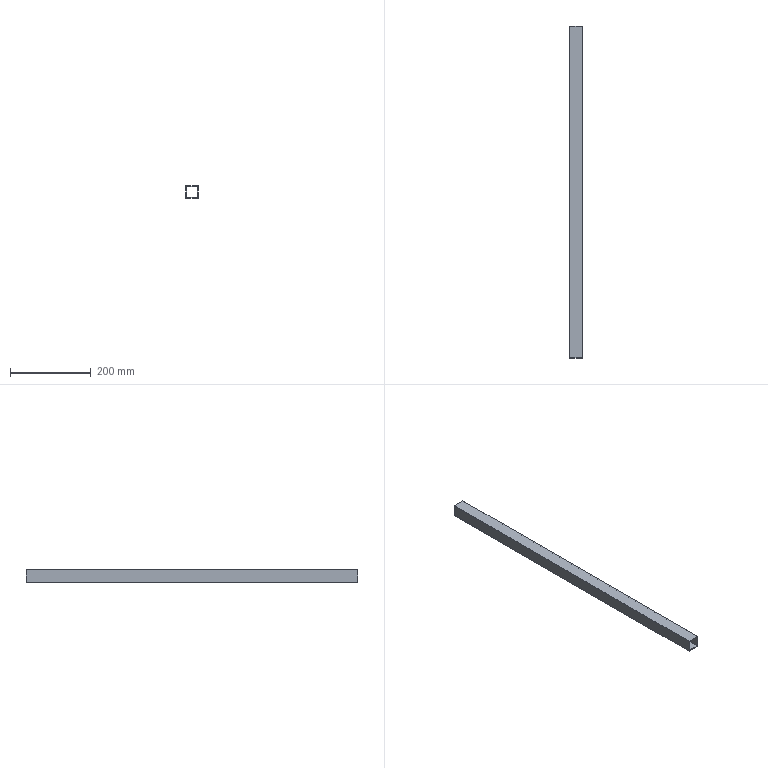Part | NX | features solid 2 | 1 solid | 10 faces | box 30 x 820 x 30 mm | volume 183680 mm3 | plane 10
STEP:
#1=CARTESIAN_POINT('',(280.,470.,50.));
#2=VERTEX_POINT('',#1);
#3=CARTESIAN_POINT('',(280.,-350.,50.));
#4=VERTEX_POINT('',#3);
#5=CARTESIAN_POINT('',(280.,210.,50.));
#6=DIRECTION('',(0.,-1.,0.));
#7=VECTOR('',#6,1000.);
#8=LINE('',#5,#7);
#9=EDGE_CURVE('',#2,#4,#8,.T.);
#10=ORIENTED_EDGE('',*,*,#9,.T.);
#11=CARTESIAN_POINT('',(280.,-350.,20.));
#12=VERTEX_POINT('',#11);
#13=CARTESIAN_POINT('',(280.,-350.,50.));
#14=DIRECTION('',(0.,0.,-1.));
#15=VECTOR('',#14,1000.);
#16=LINE('',#13,#15);
#17=EDGE_CURVE('',#4,#12,#16,.T.);
#18=ORIENTED_EDGE('',*,*,#17,.T.);
#19=CARTESIAN_POINT('',(280.,470.,20.));
#20=VERTEX_POINT('',#19);
#21=CARTESIAN_POINT('',(280.,210.,20.));
#22=DIRECTION('',(0.,-1.,0.));
#23=VECTOR('',#22,1000.);
#24=LINE('',#21,#23);
#25=EDGE_CURVE('',#20,#12,#24,.T.);
#26=ORIENTED_EDGE('',*,*,#25,.F.);
#27=CARTESIAN_POINT('',(280.,470.,50.));
#28=DIRECTION('',(0.,0.,-1.));
#29=VECTOR('',#28,1000.);
#30=LINE('',#27,#29);
#31=EDGE_CURVE('',#2,#20,#30,.T.);
#32=ORIENTED_EDGE('',*,*,#31,.F.);
#33=EDGE_LOOP('',(#10,#18,#26,#32));
#34=FACE_BOUND('',#33,.T.);
#35=CARTESIAN_POINT('',(280.,210.,50.));
#36=DIRECTION('',(1.,0.,0.));
#37=DIRECTION('',(0.,0.,-1.));
#38=AXIS2_PLACEMENT_3D('',#35,#36,#37);
#39=PLANE('',#38);
#40=ADVANCED_FACE('',(#34),#39,.T.);
#41=CARTESIAN_POINT('',(250.,-350.,50.));
#42=VERTEX_POINT('',#41);
#43=CARTESIAN_POINT('',(250.,-350.,20.));
#44=VERTEX_POINT('',#43);
#45=CARTESIAN_POINT('',(250.,-350.,50.));
#46=DIRECTION('',(0.,0.,-1.));
#47=VECTOR('',#46,1000.);
#48=LINE('',#45,#47);
#49=EDGE_CURVE('',#42,#44,#48,.T.);
#50=ORIENTED_EDGE('',*,*,#49,.F.);
#51=CARTESIAN_POINT('',(250.,470.,50.));
#52=VERTEX_POINT('',#51);
#53=CARTESIAN_POINT('',(250.,210.,50.));
#54=DIRECTION('',(0.,-1.,0.));
#55=VECTOR('',#54,1000.);
#56=LINE('',#53,#55);
#57=EDGE_CURVE('',#52,#42,#56,.T.);
#58=ORIENTED_EDGE('',*,*,#57,.F.);
#59=CARTESIAN_POINT('',(250.,470.,20.));
#60=VERTEX_POINT('',#59);
#61=CARTESIAN_POINT('',(250.,470.,50.));
#62=DIRECTION('',(0.,0.,-1.));
#63=VECTOR('',#62,1000.);
#64=LINE('',#61,#63);
#65=EDGE_CURVE('',#52,#60,#64,.T.);
#66=ORIENTED_EDGE('',*,*,#65,.T.);
#67=CARTESIAN_POINT('',(250.,210.,20.));
#68=DIRECTION('',(0.,-1.,0.));
#69=VECTOR('',#68,1000.);
#70=LINE('',#67,#69);
#71=EDGE_CURVE('',#60,#44,#70,.T.);
#72=ORIENTED_EDGE('',*,*,#71,.T.);
#73=EDGE_LOOP('',(#50,#58,#66,#72));
#74=FACE_BOUND('',#73,.T.);
#75=CARTESIAN_POINT('',(250.,210.,50.));
#76=DIRECTION('',(1.,0.,0.));
#77=DIRECTION('',(0.,0.,-1.));
#78=AXIS2_PLACEMENT_3D('',#75,#76,#77);
#79=PLANE('',#78);
#80=ADVANCED_FACE('',(#74),#79,.F.);
#81=CARTESIAN_POINT('',(280.,-350.,50.));
#82=DIRECTION('',(-1.,0.,0.));
#83=VECTOR('',#82,1000.);
#84=LINE('',#81,#83);
#85=EDGE_CURVE('',#4,#42,#84,.T.);
#86=ORIENTED_EDGE('',*,*,#85,.F.);
#87=ORIENTED_EDGE('',*,*,#9,.F.);
#88=CARTESIAN_POINT('',(280.,470.,50.));
#89=DIRECTION('',(1.,0.,0.));
#90=VECTOR('',#89,1000.);
#91=LINE('',#88,#90);
#92=EDGE_CURVE('',#52,#2,#91,.T.);
#93=ORIENTED_EDGE('',*,*,#92,.F.);
#94=ORIENTED_EDGE('',*,*,#57,.T.);
#95=EDGE_LOOP('',(#86,#87,#93,#94));
#96=FACE_BOUND('',#95,.T.);
#97=CARTESIAN_POINT('',(280.,210.,50.));
#98=DIRECTION('',(0.,0.,-1.));
#99=DIRECTION('',(-1.,0.,0.));
#100=AXIS2_PLACEMENT_3D('',#97,#98,#99);
#101=PLANE('',#100);
#102=ADVANCED_FACE('',(#96),#101,.F.);
#103=ORIENTED_EDGE('',*,*,#25,.T.);
#104=CARTESIAN_POINT('',(280.,-350.,20.));
#105=DIRECTION('',(-1.,0.,0.));
#106=VECTOR('',#105,1000.);
#107=LINE('',#104,#106);
#108=EDGE_CURVE('',#12,#44,#107,.T.);
#109=ORIENTED_EDGE('',*,*,#108,.T.);
#110=ORIENTED_EDGE('',*,*,#71,.F.);
#111=CARTESIAN_POINT('',(280.,470.,20.));
#112=DIRECTION('',(1.,0.,0.));
#113=VECTOR('',#112,1000.);
#114=LINE('',#111,#113);
#115=EDGE_CURVE('',#60,#20,#114,.T.);
#116=ORIENTED_EDGE('',*,*,#115,.T.);
#117=EDGE_LOOP('',(#103,#109,#110,#116));
#118=FACE_BOUND('',#117,.T.);
#119=CARTESIAN_POINT('',(280.,210.,20.));
#120=DIRECTION('',(0.,0.,-1.));
#121=DIRECTION('',(-1.,0.,0.));
#122=AXIS2_PLACEMENT_3D('',#119,#120,#121);
#123=PLANE('',#122);
#124=ADVANCED_FACE('',(#118),#123,.T.);
#125=CARTESIAN_POINT('',(278.,-350.,48.));
#126=VERTEX_POINT('',#125);
#127=CARTESIAN_POINT('',(278.,-350.,22.));
#128=VERTEX_POINT('',#127);
#129=CARTESIAN_POINT('',(278.,-350.,50.));
#130=DIRECTION('',(0.,0.,-1.));
#131=VECTOR('',#130,1000.);
#132=LINE('',#129,#131);
#133=EDGE_CURVE('',#126,#128,#132,.T.);
#134=ORIENTED_EDGE('',*,*,#133,.F.);
#135=CARTESIAN_POINT('',(278.,470.,48.));
#136=VERTEX_POINT('',#135);
#137=CARTESIAN_POINT('',(278.,210.,48.));
#138=DIRECTION('',(0.,-1.,0.));
#139=VECTOR('',#138,1000.);
#140=LINE('',#137,#139);
#141=EDGE_CURVE('',#136,#126,#140,.T.);
#142=ORIENTED_EDGE('',*,*,#141,.F.);
#143=CARTESIAN_POINT('',(278.,470.,22.));
#144=VERTEX_POINT('',#143);
#145=CARTESIAN_POINT('',(278.,470.,50.));
#146=DIRECTION('',(0.,0.,-1.));
#147=VECTOR('',#146,1000.);
#148=LINE('',#145,#147);
#149=EDGE_CURVE('',#136,#144,#148,.T.);
#150=ORIENTED_EDGE('',*,*,#149,.T.);
#151=CARTESIAN_POINT('',(278.,210.,22.));
#152=DIRECTION('',(0.,-1.,0.));
#153=VECTOR('',#152,1000.);
#154=LINE('',#151,#153);
#155=EDGE_CURVE('',#144,#128,#154,.T.);
#156=ORIENTED_EDGE('',*,*,#155,.T.);
#157=EDGE_LOOP('',(#134,#142,#150,#156));
#158=FACE_BOUND('',#157,.T.);
#159=CARTESIAN_POINT('',(278.,210.,50.));
#160=DIRECTION('',(1.,0.,0.));
#161=DIRECTION('',(0.,0.,-1.));
#162=AXIS2_PLACEMENT_3D('',#159,#160,#161);
#163=PLANE('',#162);
#164=ADVANCED_FACE('',(#158),#163,.F.);
#165=CARTESIAN_POINT('',(252.,470.,48.));
#166=VERTEX_POINT('',#165);
#167=CARTESIAN_POINT('',(252.,-350.,48.));
#168=VERTEX_POINT('',#167);
#169=CARTESIAN_POINT('',(252.,210.,48.));
#170=DIRECTION('',(0.,-1.,0.));
#171=VECTOR('',#170,1000.);
#172=LINE('',#169,#171);
#173=EDGE_CURVE('',#166,#168,#172,.T.);
#174=ORIENTED_EDGE('',*,*,#173,.T.);
#175=CARTESIAN_POINT('',(252.,-350.,22.));
#176=VERTEX_POINT('',#175);
#177=CARTESIAN_POINT('',(252.,-350.,50.));
#178=DIRECTION('',(0.,0.,-1.));
#179=VECTOR('',#178,1000.);
#180=LINE('',#177,#179);
#181=EDGE_CURVE('',#168,#176,#180,.T.);
#182=ORIENTED_EDGE('',*,*,#181,.T.);
#183=CARTESIAN_POINT('',(252.,470.,22.));
#184=VERTEX_POINT('',#183);
#185=CARTESIAN_POINT('',(252.,210.,22.));
#186=DIRECTION('',(0.,-1.,0.));
#187=VECTOR('',#186,1000.);
#188=LINE('',#185,#187);
#189=EDGE_CURVE('',#184,#176,#188,.T.);
#190=ORIENTED_EDGE('',*,*,#189,.F.);
#191=CARTESIAN_POINT('',(252.,470.,50.));
#192=DIRECTION('',(0.,0.,-1.));
#193=VECTOR('',#192,1000.);
#194=LINE('',#191,#193);
#195=EDGE_CURVE('',#166,#184,#194,.T.);
#196=ORIENTED_EDGE('',*,*,#195,.F.);
#197=EDGE_LOOP('',(#174,#182,#190,#196));
#198=FACE_BOUND('',#197,.T.);
#199=CARTESIAN_POINT('',(252.,210.,50.));
#200=DIRECTION('',(1.,0.,0.));
#201=DIRECTION('',(0.,0.,-1.));
#202=AXIS2_PLACEMENT_3D('',#199,#200,#201);
#203=PLANE('',#202);
#204=ADVANCED_FACE('',(#198),#203,.T.);
#205=ORIENTED_EDGE('',*,*,#141,.T.);
#206=CARTESIAN_POINT('',(280.,-350.,48.));
#207=DIRECTION('',(-1.,0.,0.));
#208=VECTOR('',#207,1000.);
#209=LINE('',#206,#208);
#210=EDGE_CURVE('',#126,#168,#209,.T.);
#211=ORIENTED_EDGE('',*,*,#210,.T.);
#212=ORIENTED_EDGE('',*,*,#173,.F.);
#213=CARTESIAN_POINT('',(280.,470.,48.));
#214=DIRECTION('',(1.,0.,0.));
#215=VECTOR('',#214,1000.);
#216=LINE('',#213,#215);
#217=EDGE_CURVE('',#166,#136,#216,.T.);
#218=ORIENTED_EDGE('',*,*,#217,.T.);
#219=EDGE_LOOP('',(#205,#211,#212,#218));
#220=FACE_BOUND('',#219,.T.);
#221=CARTESIAN_POINT('',(280.,210.,48.));
#222=DIRECTION('',(0.,0.,-1.));
#223=DIRECTION('',(-1.,0.,0.));
#224=AXIS2_PLACEMENT_3D('',#221,#222,#223);
#225=PLANE('',#224);
#226=ADVANCED_FACE('',(#220),#225,.T.);
#227=CARTESIAN_POINT('',(280.,-350.,22.));
#228=DIRECTION('',(-1.,0.,0.));
#229=VECTOR('',#228,1000.);
#230=LINE('',#227,#229);
#231=EDGE_CURVE('',#128,#176,#230,.T.);
#232=ORIENTED_EDGE('',*,*,#231,.F.);
#233=ORIENTED_EDGE('',*,*,#155,.F.);
#234=CARTESIAN_POINT('',(280.,470.,22.));
#235=DIRECTION('',(1.,0.,0.));
#236=VECTOR('',#235,1000.);
#237=LINE('',#234,#236);
#238=EDGE_CURVE('',#184,#144,#237,.T.);
#239=ORIENTED_EDGE('',*,*,#238,.F.);
#240=ORIENTED_EDGE('',*,*,#189,.T.);
#241=EDGE_LOOP('',(#232,#233,#239,#240));
#242=FACE_BOUND('',#241,.T.);
#243=CARTESIAN_POINT('',(280.,210.,22.));
#244=DIRECTION('',(0.,0.,-1.));
#245=DIRECTION('',(-1.,0.,0.));
#246=AXIS2_PLACEMENT_3D('',#243,#244,#245);
#247=PLANE('',#246);
#248=ADVANCED_FACE('',(#242),#247,.F.);
#249=ORIENTED_EDGE('',*,*,#115,.F.);
#250=ORIENTED_EDGE('',*,*,#65,.F.);
#251=ORIENTED_EDGE('',*,*,#92,.T.);
#252=ORIENTED_EDGE('',*,*,#31,.T.);
#253=EDGE_LOOP('',(#249,#250,#251,#252));
#254=FACE_BOUND('',#253,.T.);
#255=ORIENTED_EDGE('',*,*,#195,.T.);
#256=ORIENTED_EDGE('',*,*,#238,.T.);
#257=ORIENTED_EDGE('',*,*,#149,.F.);
#258=ORIENTED_EDGE('',*,*,#217,.F.);
#259=EDGE_LOOP('',(#255,#256,#257,#258));
#260=FACE_BOUND('',#259,.T.);
#261=CARTESIAN_POINT('',(-240.,470.,50.));
#262=DIRECTION('',(0.,1.,0.));
#263=DIRECTION('',(0.,0.,1.));
#264=AXIS2_PLACEMENT_3D('',#261,#262,#263);
#265=PLANE('',#264);
#266=ADVANCED_FACE('',(#254,#260),#265,.T.);
#267=ORIENTED_EDGE('',*,*,#210,.F.);
#268=ORIENTED_EDGE('',*,*,#133,.T.);
#269=ORIENTED_EDGE('',*,*,#231,.T.);
#270=ORIENTED_EDGE('',*,*,#181,.F.);
#271=EDGE_LOOP('',(#267,#268,#269,#270));
#272=FACE_BOUND('',#271,.T.);
#273=ORIENTED_EDGE('',*,*,#17,.F.);
#274=ORIENTED_EDGE('',*,*,#85,.T.);
#275=ORIENTED_EDGE('',*,*,#49,.T.);
#276=ORIENTED_EDGE('',*,*,#108,.F.);
#277=EDGE_LOOP('',(#273,#274,#275,#276));
#278=FACE_BOUND('',#277,.T.);
#279=CARTESIAN_POINT('',(250.,-350.,50.));
#280=DIRECTION('',(0.,-1.,0.));
#281=DIRECTION('',(0.,0.,-1.));
#282=AXIS2_PLACEMENT_3D('',#279,#280,#281);
#283=PLANE('',#282);
#284=ADVANCED_FACE('',(#272,#278),#283,.T.);
#285=CLOSED_SHELL('',(#40,#80,#102,#124,#164,#204,#226,#248,#266,#284));
#286=MANIFOLD_SOLID_BREP('',#285);
#287=(LENGTH_UNIT()NAMED_UNIT(*)SI_UNIT(.MILLI.,.METRE.));
#288=UNCERTAINTY_MEASURE_WITH_UNIT(LENGTH_MEASURE(0.00001),#287,'','');
#289=(NAMED_UNIT(*)PLANE_ANGLE_UNIT()SI_UNIT($,.RADIAN.));
#290=(NAMED_UNIT(*)SI_UNIT($,.STERADIAN.)SOLID_ANGLE_UNIT());
#291=(GEOMETRIC_REPRESENTATION_CONTEXT(3)GLOBAL_UNCERTAINTY_ASSIGNED_CONTEXT((#288))GLOBAL_UNIT_ASSIGNED_CONTEXT((#287,#289,#290))REPRESENTATION_CONTEXT('',''));
#292=ADVANCED_BREP_SHAPE_REPRESENTATION('',(#286),#291);